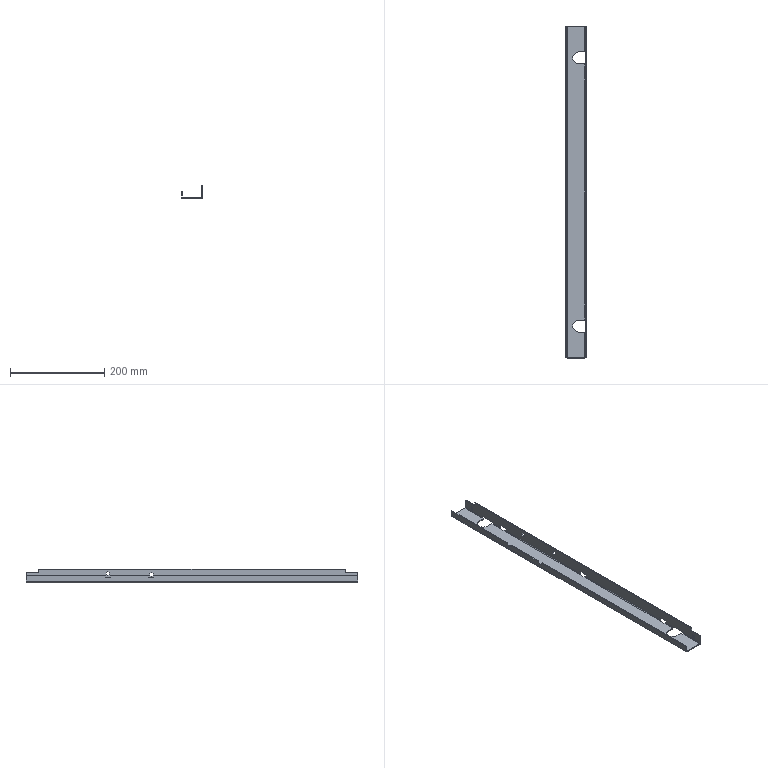Part | STEP file | Lower door gasket strip vertical (door lock) modified | 1 solid | 105 faces | box 44.5 x 705 x 28.5 mm | volume 109938 mm3 | plane 83 | cylinder 22 | commonest cylinder face diameters 3 x9 7 x9 25 x4